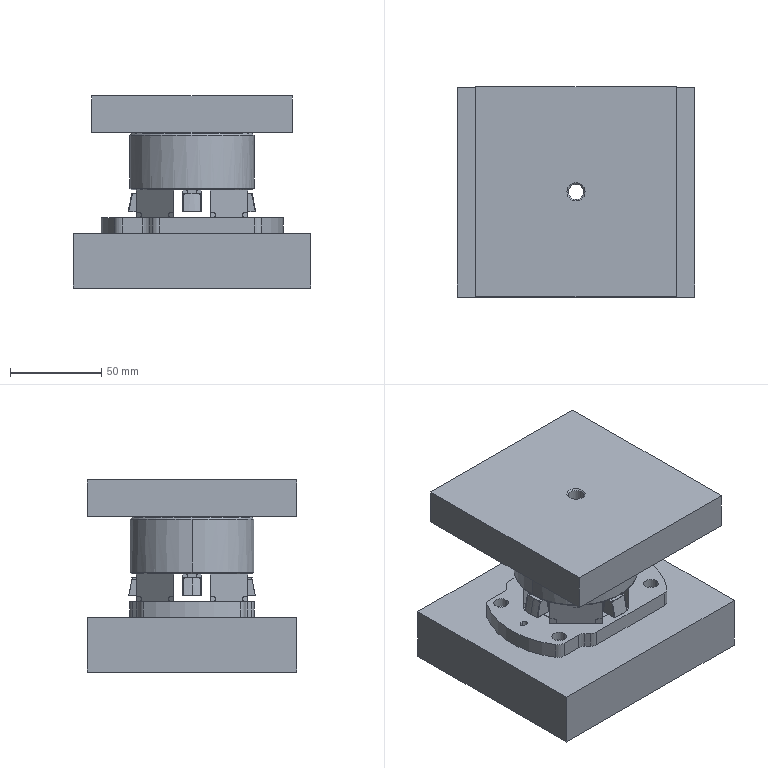NC program | NX | posted with a generic post | part box 130 x 115 x 105.2 mm
Lines 1 to 1155 of 3719:
N10 G17 G21 G94 G90
(PLANAR_MILL_COPY_4 , TOOL : D1.5R0)
N12 T16 M6
N14 G54
N16 G17 G0 G90 X-2.302 Y-5.448 S6000 M3
N18 G43 Z94. H16
N20 G94 G1 Z34.46 F5000.
N22 G41 X-3.284 Y-5.258 F1400. D16
N24 X-3.371 Y-5.25
N26 X-10.443
N28 X-12.2
N30 G2 X-13.95 Y-3.5 R1.75
N32 G3 X-14.2 Y-3.25 R0.25
N34 X-14.45 Y-3.5 R0.25
N36 G1 Y-4.929
N38 X-14.442 Y-5.016
N40 G40
N42 X-14.252 Y-5.998
N44 G0 Z37.71
N46 X-2.302 Y-5.448
N48 G1 Z34.21 F5000.
N50 G41 X-3.284 Y-5.258 F1400.
N52 X-3.371 Y-5.25
N54 X-10.443
N56 X-12.2
N58 G2 X-13.95 Y-3.5 R1.75
N60 G3 X-14.2 Y-3.25 R0.25
N62 X-14.45 Y-3.5 R0.25
N64 G1 Y-4.929
N66 X-14.442 Y-5.016
N68 G40
N70 X-14.252 Y-5.998
N72 G0 Z37.71
N74 X-2.302 Y-5.448
N76 G1 Z33.96 F5000.
N78 G41 X-3.284 Y-5.258 F1400.
N80 X-3.371 Y-5.25
N82 X-10.443
N84 X-12.2
N86 G2 X-13.95 Y-3.5 R1.75
N88 G3 X-14.2 Y-3.25 R0.25
N90 X-14.45 Y-3.5 R0.25
N92 G1 Y-4.929
N94 X-14.442 Y-5.016
N96 G40
N98 X-14.252 Y-5.998
N100 G0 Z37.71
N102 X-2.302 Y-5.448
N104 G1 Z33.71 F5000.
N106 G41 X-3.284 Y-5.258 F1400.
N108 X-3.371 Y-5.25
N110 X-10.443
N112 X-12.2
N114 G2 X-13.95 Y-3.5 R1.75
N116 G3 X-14.2 Y-3.25 R0.25
N118 X-14.45 Y-3.5 R0.25
N120 G1 Y-4.929
N122 X-14.442 Y-5.016
N124 G40
N126 X-14.252 Y-5.998
N128 G0 Z37.71
N130 X-2.302 Y-5.448
N132 G1 Z33.46 F5000.
N134 G41 X-3.284 Y-5.258 F1400.
N136 X-3.371 Y-5.25
N138 X-10.443
N140 X-12.2
N142 G2 X-13.95 Y-3.5 R1.75
N144 G3 X-14.2 Y-3.25 R0.25
N146 X-14.45 Y-3.5 R0.25
N148 G1 Y-4.929
N150 X-14.442 Y-5.016
N152 G40
N154 X-14.252 Y-5.998
N156 G0 Z37.71
N158 X-2.302 Y-5.448
N160 G1 Z33.21 F5000.
N162 G41 X-3.284 Y-5.258 F1400.
N164 X-3.371 Y-5.25
N166 X-10.443
N168 X-12.2
N170 G2 X-13.95 Y-3.5 R1.75
N172 G3 X-14.2 Y-3.25 R0.25
N174 X-14.45 Y-3.5 R0.25
N176 G1 Y-4.929
N178 X-14.442 Y-5.016
N180 G40
N182 X-14.252 Y-5.998
N184 G0 Z37.71
N186 X-2.302 Y-5.448
N188 G1 Z32.96 F5000.
N190 G41 X-3.284 Y-5.258 F1400.
N192 X-3.371 Y-5.25
N194 X-10.443
N196 X-12.2
N198 G2 X-13.95 Y-3.5 R1.75
N200 G3 X-14.2 Y-3.25 R0.25
N202 X-14.45 Y-3.5 R0.25
N204 G1 Y-4.929
N206 X-14.442 Y-5.016
N208 G40
N210 X-14.252 Y-5.998
N212 G0 Z37.71
N214 X-2.302 Y-5.448
N216 G1 Z32.71 F5000.
N218 G41 X-3.284 Y-5.258 F1400.
N220 X-3.371 Y-5.25
N222 X-10.443
N224 X-12.2
N226 G2 X-13.95 Y-3.5 R1.75
N228 G3 X-14.2 Y-3.25 R0.25
N230 X-14.45 Y-3.5 R0.25
N232 G1 Y-4.929
N234 X-14.442 Y-5.016
N236 G40
N238 X-14.252 Y-5.998
N240 G0 Z37.71
N242 X-2.302 Y-5.448
N244 G1 Z32.46 F5000.
N246 G41 X-3.284 Y-5.258 F1400.
N248 X-3.371 Y-5.25
N250 X-10.443
N252 X-12.2
N254 G2 X-13.95 Y-3.5 R1.75
N256 G3 X-14.2 Y-3.25 R0.25
N258 X-14.45 Y-3.5 R0.25
N260 G1 Y-4.929
N262 X-14.442 Y-5.016
N264 G40
N266 X-14.252 Y-5.998
N268 G0 Z37.71
N270 X-2.302 Y-5.448
N272 G1 Z32.21 F5000.
N274 G41 X-3.284 Y-5.258 F1400.
N276 X-3.371 Y-5.25
N278 X-10.443
N280 X-12.2
N282 G2 X-13.95 Y-3.5 R1.75
N284 G3 X-14.2 Y-3.25 R0.25
N286 X-14.45 Y-3.5 R0.25
N288 G1 Y-4.929
N290 X-14.442 Y-5.016
N292 G40
N294 X-14.252 Y-5.998
N296 G0 Z37.71
N298 X-2.302 Y-5.448
N300 G1 Z31.96 F5000.
N302 G41 X-3.284 Y-5.258 F1400.
N304 X-3.371 Y-5.25
N306 X-10.443
N308 X-12.2
N310 G2 X-13.95 Y-3.5 R1.75
N312 G3 X-14.2 Y-3.25 R0.25
N314 X-14.45 Y-3.5 R0.25
N316 G1 Y-4.929
N318 X-14.442 Y-5.016
N320 G40
N322 X-14.252 Y-5.998
N324 G0 Z37.71
N326 X-2.302 Y-5.448
N328 G1 Z31.71 F5000.
N330 G41 X-3.284 Y-5.258 F1400.
N332 X-3.371 Y-5.25
N334 X-10.443
N336 X-12.2
N338 G2 X-13.95 Y-3.5 R1.75
N340 G3 X-14.2 Y-3.25 R0.25
N342 X-14.45 Y-3.5 R0.25
N344 G1 Y-4.929
N346 X-14.442 Y-5.016
N348 G40
N350 X-14.252 Y-5.998
N352 G0 Z37.71
N354 X-2.302 Y-5.448
N356 G1 Z31.46 F5000.
N358 G41 X-3.284 Y-5.258 F1400.
N360 X-3.371 Y-5.25
N362 X-10.443
N364 X-12.2
N366 G2 X-13.95 Y-3.5 R1.75
N368 G3 X-14.2 Y-3.25 R0.25
N370 X-14.45 Y-3.5 R0.25
N372 G1 Y-4.929
N374 X-14.442 Y-5.016
N376 G40
N378 X-14.252 Y-5.998
N380 G0 Z37.71
N382 X-2.302 Y-5.448
N384 G1 Z31.21 F5000.
N386 G41 X-3.284 Y-5.258 F1400.
N388 X-3.371 Y-5.25
N390 X-10.443
N392 X-12.2
N394 G2 X-13.95 Y-3.5 R1.75
N396 G3 X-14.2 Y-3.25 R0.25
N398 X-14.45 Y-3.5 R0.25
N400 G1 Y-4.929
N402 X-14.442 Y-5.016
N404 G40
N406 X-14.252 Y-5.998
N408 G0 Z37.71
N410 X-2.302 Y-5.448
N412 G1 Z30.96 F5000.
N414 G41 X-3.284 Y-5.258 F1400.
N416 X-3.371 Y-5.25
N418 X-10.443
N420 X-12.2
N422 G2 X-13.95 Y-3.5 R1.75
N424 G3 X-14.2 Y-3.25 R0.25
N426 X-14.45 Y-3.5 R0.25
N428 G1 Y-4.929
N430 X-14.442 Y-5.016
N432 G40
N434 X-14.252 Y-5.998
N436 G0 Z37.71
N438 X-2.302 Y-5.448
N440 G1 Z30.71 F5000.
N442 G41 X-3.284 Y-5.258 F1400.
N444 X-3.371 Y-5.25
N446 X-10.443
N448 X-12.2
N450 G2 X-13.95 Y-3.5 R1.75
N452 G3 X-14.2 Y-3.25 R0.25
N454 X-14.45 Y-3.5 R0.25
N456 G1 Y-4.929
N458 X-14.442 Y-5.016
N460 G40
N462 X-14.252 Y-5.998
N464 G0 Z37.71
N466 X-2.302 Y-5.448
N468 G1 Z30.46 F5000.
N470 G41 X-3.284 Y-5.258 F1400.
N472 X-3.371 Y-5.25
N474 X-10.443
N476 X-12.2
N478 G2 X-13.95 Y-3.5 R1.75
N480 G3 X-14.2 Y-3.25 R0.25
N482 X-14.45 Y-3.5 R0.25
N484 G1 Y-4.929
N486 X-14.442 Y-5.016
N488 G40
N490 X-14.252 Y-5.998
N492 G0 Z37.71
N494 X-2.302 Y-5.448
N496 G1 Z30.21 F5000.
N498 G41 X-3.284 Y-5.258 F1400.
N500 X-3.371 Y-5.25
N502 X-10.443
N504 X-12.2
N506 G2 X-13.95 Y-3.5 R1.75
N508 G3 X-14.2 Y-3.25 R0.25
N510 X-14.45 Y-3.5 R0.25
N512 G1 Y-4.929
N514 X-14.442 Y-5.016
N516 G40
N518 X-14.252 Y-5.998
N520 G0 Z37.71
N522 X-2.302 Y-5.448
N524 G1 Z29.96 F5000.
N526 G41 X-3.284 Y-5.258 F1400.
N528 X-3.371 Y-5.25
N530 X-10.443
N532 X-12.2
N534 G2 X-13.95 Y-3.5 R1.75
N536 G3 X-14.2 Y-3.25 R0.25
N538 X-14.45 Y-3.5 R0.25
N540 G1 Y-4.929
N542 X-14.442 Y-5.016
N544 G40
N546 X-14.252 Y-5.998
N548 G0 Z37.71
N550 X-2.302 Y-5.448
N552 G1 Z29.71 F5000.
N554 G41 X-3.284 Y-5.258 F1400.
N556 X-3.371 Y-5.25
N558 X-10.443
N560 X-12.2
N562 G2 X-13.95 Y-3.5 R1.75
N564 G3 X-14.2 Y-3.25 R0.25
N566 X-14.45 Y-3.5 R0.25
N568 G1 Y-4.929
N570 X-14.442 Y-5.016
N572 G40
N574 X-14.252 Y-5.998
N576 G0 Z37.71
N578 X-2.302 Y-5.448
N580 G1 Z29.46 F5000.
N582 G41 X-3.284 Y-5.258 F1400.
N584 X-3.371 Y-5.25
N586 X-10.443
N588 X-12.2
N590 G2 X-13.95 Y-3.5 R1.75
N592 G3 X-14.2 Y-3.25 R0.25
N594 X-14.45 Y-3.5 R0.25
N596 G1 Y-4.929
N598 X-14.442 Y-5.016
N600 G40
N602 X-14.252 Y-5.998
N604 G0 Z37.71
N606 X-2.302 Y-5.448
N608 G1 Z29.21 F5000.
N610 G41 X-3.284 Y-5.258 F1400.
N612 X-3.371 Y-5.25
N614 X-10.443
N616 X-12.2
N618 G2 X-13.95 Y-3.5 R1.75
N620 G3 X-14.2 Y-3.25 R0.25
N622 X-14.45 Y-3.5 R0.25
N624 G1 Y-4.929
N626 X-14.442 Y-5.016
N628 G40
N630 X-14.252 Y-5.998
N632 G0 Z37.71
N634 X-2.302 Y-5.448
N636 G1 Z28.96 F5000.
N638 G41 X-3.284 Y-5.258 F1400.
N640 X-3.371 Y-5.25
N642 X-10.443
N644 X-12.2
N646 G2 X-13.95 Y-3.5 R1.75
N648 G3 X-14.2 Y-3.25 R0.25
N650 X-14.45 Y-3.5 R0.25
N652 G1 Y-4.929
N654 X-14.442 Y-5.016
N656 G40
N658 X-14.252 Y-5.998
N660 G0 Z37.71
N662 X-2.302 Y-5.448
N664 G1 Z28.71 F5000.
N666 G41 X-3.284 Y-5.258 F1400.
N668 X-3.371 Y-5.25
N670 X-10.443
N672 X-12.2
N674 G2 X-13.95 Y-3.5 R1.75
N676 G3 X-14.2 Y-3.25 R0.25
N678 X-14.45 Y-3.5 R0.25
N680 G1 Y-4.929
N682 X-14.442 Y-5.016
N684 G40
N686 X-14.252 Y-5.998
N688 G0 Z37.71
N690 X-2.302 Y-5.448
N692 G1 Z28.46 F5000.
N694 G41 X-3.284 Y-5.258 F1400.
N696 X-3.371 Y-5.25
N698 X-10.443
N700 X-12.2
N702 G2 X-13.95 Y-3.5 R1.75
N704 G3 X-14.2 Y-3.25 R0.25
N706 X-14.45 Y-3.5 R0.25
N708 G1 Y-4.929
N710 X-14.442 Y-5.016
N712 G40
N714 X-14.252 Y-5.998
N716 G0 Z37.71
N718 X-2.302 Y-5.448
N720 G1 Z28.21 F5000.
N722 G41 X-3.284 Y-5.258 F1400.
N724 X-3.371 Y-5.25
N726 X-10.443
N728 X-12.2
N730 G2 X-13.95 Y-3.5 R1.75
N732 G3 X-14.2 Y-3.25 R0.25
N734 X-14.45 Y-3.5 R0.25
N736 G1 Y-4.929
N738 X-14.442 Y-5.016
N740 G40
N742 X-14.252 Y-5.998
N744 G0 Z37.71
N746 X-2.302 Y-5.448
N748 G1 Z27.96 F5000.
N750 G41 X-3.284 Y-5.258 F1400.
N752 X-3.371 Y-5.25
N754 X-10.443
N756 X-12.2
N758 G2 X-13.95 Y-3.5 R1.75
N760 G3 X-14.2 Y-3.25 R0.25
N762 X-14.45 Y-3.5 R0.25
N764 G1 Y-4.929
N766 X-14.442 Y-5.016
N768 G40
N770 X-14.252 Y-5.998
N772 G0 Z37.71
N774 X-2.302 Y-5.448
N776 G1 Z27.71 F5000.
N778 G41 X-3.284 Y-5.258 F1400.
N780 X-3.371 Y-5.25
N782 X-10.443
N784 X-12.2
N786 G2 X-13.95 Y-3.5 R1.75
N788 G3 X-14.2 Y-3.25 R0.25
N790 X-14.45 Y-3.5 R0.25
N792 G1 Y-4.929
N794 X-14.442 Y-5.016
N796 G40
N798 X-14.252 Y-5.998
N800 G0 Z37.71
N802 X-2.302 Y-5.448
N804 G1 Z27.46 F5000.
N806 G41 X-3.284 Y-5.258 F1400.
N808 X-3.371 Y-5.25
N810 X-10.443
N812 X-12.2
N814 G2 X-13.95 Y-3.5 R1.75
N816 G3 X-14.2 Y-3.25 R0.25
N818 X-14.45 Y-3.5 R0.25
N820 G1 Y-4.929
N822 X-14.442 Y-5.016
N824 G40
N826 X-14.252 Y-5.998
N828 G0 Z37.71
N830 X-2.302 Y-5.448
N832 G1 Z27.21 F5000.
N834 G41 X-3.284 Y-5.258 F1400.
N836 X-3.371 Y-5.25
N838 X-10.443
N840 X-12.2
N842 G2 X-13.95 Y-3.5 R1.75
N844 G3 X-14.2 Y-3.25 R0.25
N846 X-14.45 Y-3.5 R0.25
N848 G1 Y-4.929
N850 X-14.442 Y-5.016
N852 G40
N854 X-14.252 Y-5.998
N856 G0 Z37.71
N858 X-2.302 Y-5.448
N860 G1 Z26.96 F5000.
N862 G41 X-3.284 Y-5.258 F1400.
N864 X-3.371 Y-5.25
N866 X-10.443
N868 X-12.2
N870 G2 X-13.95 Y-3.5 R1.75
N872 G3 X-14.2 Y-3.25 R0.25
N874 X-14.45 Y-3.5 R0.25
N876 G1 Y-4.929
N878 X-14.442 Y-5.016
N880 G40
N882 X-14.252 Y-5.998
N884 G0 Z37.71
N886 X-2.302 Y-5.448
N888 G1 Z26.71 F5000.
N890 G41 X-3.284 Y-5.258 F1400.
N892 X-3.371 Y-5.25
N894 X-10.443
N896 X-12.2
N898 G2 X-13.95 Y-3.5 R1.75
N900 G3 X-14.2 Y-3.25 R0.25
N902 X-14.45 Y-3.5 R0.25
N904 G1 Y-4.929
N906 X-14.442 Y-5.016
N908 G40
N910 X-14.252 Y-5.998
N912 G0 Z37.71
N914 X-2.302 Y-5.448
N916 G1 Z26.55 F5000.
N918 G41 X-3.284 Y-5.258 F1400.
N920 X-3.371 Y-5.25
N922 X-10.443
N924 X-12.2
N926 G2 X-13.95 Y-3.5 R1.75
N928 G3 X-14.2 Y-3.25 R0.25
N930 X-14.45 Y-3.5 R0.25
N932 G1 Y-4.929
N934 X-14.442 Y-5.016
N936 G40
N938 X-14.252 Y-5.998
N940 G0 Z37.71
N942 Y5.998
N944 G1 Z34.46 F5000.
N946 G41 X-14.442 Y5.016 F1400.
N948 X-14.45 Y4.929
N950 Y3.5
N952 G3 X-14.2 Y3.25 R0.25
N954 X-13.95 Y3.5 R0.25
N956 G2 X-12.2 Y5.25 R1.75
N958 G1 X-11.317
N960 X-3.371
N962 X-3.284 Y5.258
N964 G40
N966 X-2.302 Y5.448
N968 G0 Z37.71
N970 X-14.252 Y5.998
N972 G1 Z34.21 F5000.
N974 G41 X-14.442 Y5.016 F1400.
N976 X-14.45 Y4.929
N978 Y3.5
N980 G3 X-14.2 Y3.25 R0.25
N982 X-13.95 Y3.5 R0.25
N984 G2 X-12.2 Y5.25 R1.75
N986 G1 X-11.317
N988 X-3.371
N990 X-3.284 Y5.258
N992 G40
N994 X-2.302 Y5.448
N996 G0 Z37.71
N998 X-14.252 Y5.998
N1000 G1 Z33.96 F5000.
N1002 G41 X-14.442 Y5.016 F1400.
N1004 X-14.45 Y4.929
N1006 Y3.5
N1008 G3 X-14.2 Y3.25 R0.25
N1010 X-13.95 Y3.5 R0.25
N1012 G2 X-12.2 Y5.25 R1.75
N1014 G1 X-11.317
N1016 X-3.371
N1018 X-3.284 Y5.258
N1020 G40
N1022 X-2.302 Y5.448
N1024 G0 Z37.71
N1026 X-14.252 Y5.998
N1028 G1 Z33.71 F5000.
N1030 G41 X-14.442 Y5.016 F1400.
N1032 X-14.45 Y4.929
N1034 Y3.5
N1036 G3 X-14.2 Y3.25 R0.25
N1038 X-13.95 Y3.5 R0.25
N1040 G2 X-12.2 Y5.25 R1.75
N1042 G1 X-11.317
N1044 X-3.371
N1046 X-3.284 Y5.258
N1048 G40
N1050 X-2.302 Y5.448
N1052 G0 Z37.71
N1054 X-14.252 Y5.998
N1056 G1 Z33.46 F5000.
N1058 G41 X-14.442 Y5.016 F1400.
N1060 X-14.45 Y4.929
N1062 Y3.5
N1064 G3 X-14.2 Y3.25 R0.25
N1066 X-13.95 Y3.5 R0.25
N1068 G2 X-12.2 Y5.25 R1.75
N1070 G1 X-11.317
N1072 X-3.371
N1074 X-3.284 Y5.258
N1076 G40
N1078 X-2.302 Y5.448
N1080 G0 Z37.71
N1082 X-14.252 Y5.998
N1084 G1 Z33.21 F5000.
N1086 G41 X-14.442 Y5.016 F1400.
N1088 X-14.45 Y4.929
N1090 Y3.5
N1092 G3 X-14.2 Y3.25 R0.25
N1094 X-13.95 Y3.5 R0.25
N1096 G2 X-12.2 Y5.25 R1.75
N1098 G1 X-11.317
N1100 X-3.371
N1102 X-3.284 Y5.258
N1104 G40
N1106 X-2.302 Y5.448
N1108 G0 Z37.71
N1110 X-14.252 Y5.998
N1112 G1 Z32.96 F5000.
N1114 G41 X-14.442 Y5.016 F1400.
N1116 X-14.45 Y4.929
N1118 Y3.5
N1120 G3 X-14.2 Y3.25 R0.25
N1122 X-13.95 Y3.5 R0.25
N1124 G2 X-12.2 Y5.25 R1.75
N1126 G1 X-11.317
N1128 X-3.371
N1130 X-3.284 Y5.258
N1132 G40
N1134 X-2.302 Y5.448
N1136 G0 Z37.71
N1138 X-14.252 Y5.998
N1140 G1 Z32.71 F5000.
N1142 G41 X-14.442 Y5.016 F1400.
N1144 X-14.45 Y4.929
N1146 Y3.5
N1148 G3 X-14.2 Y3.25 R0.25
N1150 X-13.95 Y3.5 R0.25
N1152 G2 X-12.2 Y5.25 R1.75
N1154 G1 X-11.317
N1156 X-3.371
N1158 X-3.284 Y5.258
N1160 G40
N1162 X-2.302 Y5.448
N1164 G0 Z37.71
N1166 X-14.252 Y5.998
N1168 G1 Z32.46 F5000.
N1170 G41 X-14.442 Y5.016 F1400.
N1172 X-14.45 Y4.929
N1174 Y3.5
N1176 G3 X-14.2 Y3.25 R0.25
N1178 X-13.95 Y3.5 R0.25
N1180 G2 X-12.2 Y5.25 R1.75
N1182 G1 X-11.317
N1184 X-3.371
N1186 X-3.284 Y5.258
N1188 G40
N1190 X-2.302 Y5.448
N1192 G0 Z37.71
N1194 X-14.252 Y5.998
N1196 G1 Z32.21 F5000.
N1198 G41 X-14.442 Y5.016 F1400.
N1200 X-14.45 Y4.929
N1202 Y3.5
N1204 G3 X-14.2 Y3.25 R0.25
N1206 X-13.95 Y3.5 R0.25
N1208 G2 X-12.2 Y5.25 R1.75
N1210 G1 X-11.317
N1212 X-3.371
N1214 X-3.284 Y5.258
N1216 G40
N1218 X-2.302 Y5.448
N1220 G0 Z37.71
N1222 X-14.252 Y5.998
N1224 G1 Z31.96 F5000.
N1226 G41 X-14.442 Y5.016 F1400.
N1228 X-14.45 Y4.929
N1230 Y3.5
N1232 G3 X-14.2 Y3.25 R0.25
N1234 X-13.95 Y3.5 R0.25
N1236 G2 X-12.2 Y5.25 R1.75
N1238 G1 X-11.317
N1240 X-3.371
N1242 X-3.284 Y5.258
N1244 G40
N1246 X-2.302 Y5.448
N1248 G0 Z37.71
N1250 X-14.252 Y5.998
N1252 G1 Z31.71 F5000.
N1254 G41 X-14.442 Y5.016 F1400.
N1256 X-14.45 Y4.929
N1258 Y3.5
N1260 G3 X-14.2 Y3.25 R0.25
N1262 X-13.95 Y3.5 R0.25
N1264 G2 X-12.2 Y5.25 R1.75
N1266 G1 X-11.317
N1268 X-3.371
N1270 X-3.284 Y5.258
N1272 G40
N1274 X-2.302 Y5.448
N1276 G0 Z37.71
N1278 X-14.252 Y5.998
N1280 G1 Z31.46 F5000.
N1282 G41 X-14.442 Y5.016 F1400.
N1284 X-14.45 Y4.929
N1286 Y3.5
N1288 G3 X-14.2 Y3.25 R0.25
N1290 X-13.95 Y3.5 R0.25
N1292 G2 X-12.2 Y5.25 R1.75
N1294 G1 X-11.317
N1296 X-3.371
N1298 X-3.284 Y5.258
N1300 G40
N1302 X-2.302 Y5.448
N1304 G0 Z37.71
N1306 X-14.252 Y5.998
N1308 G1 Z31.21 F5000.
N1310 G41 X-14.442 Y5.016 F1400.
N1312 X-14.45 Y4.929
N1314 Y3.5
N1316 G3 X-14.2 Y3.25 R0.25
N1318 X-13.95 Y3.5 R0.25
N1320 G2 X-12.2 Y5.25 R1.75
N1322 G1 X-11.317
N1324 X-3.371
N1326 X-3.284 Y5.258
N1328 G40
N1330 X-2.302 Y5.448
N1332 G0 Z37.71
N1334 X-14.252 Y5.998
N1336 G1 Z30.96 F5000.
N1338 G41 X-14.442 Y5.016 F1400.
N1340 X-14.45 Y4.929
N1342 Y3.5
N1344 G3 X-14.2 Y3.25 R0.25
N1346 X-13.95 Y3.5 R0.25
N1348 G2 X-12.2 Y5.25 R1.75
N1350 G1 X-11.317
N1352 X-3.371
N1354 X-3.284 Y5.258
N1356 G40
N1358 X-2.302 Y5.448
N1360 G0 Z37.71
N1362 X-14.252 Y5.998
N1364 G1 Z30.71 F5000.
N1366 G41 X-14.442 Y5.016 F1400.
N1368 X-14.45 Y4.929
N1370 Y3.5
N1372 G3 X-14.2 Y3.25 R0.25
N1374 X-13.95 Y3.5 R0.25
N1376 G2 X-12.2 Y5.25 R1.75
N1378 G1 X-11.317
N1380 X-3.371
N1382 X-3.284 Y5.258
N1384 G40
N1386 X-2.302 Y5.448
N1388 G0 Z37.71
N1390 X-14.252 Y5.998
N1392 G1 Z30.46 F5000.
N1394 G41 X-14.442 Y5.016 F1400.
N1396 X-14.45 Y4.929
N1398 Y3.5
N1400 G3 X-14.2 Y3.25 R0.25
N1402 X-13.95 Y3.5 R0.25
N1404 G2 X-12.2 Y5.25 R1.75
N1406 G1 X-11.317
N1408 X-3.371
N1410 X-3.284 Y5.258
N1412 G40
N1414 X-2.302 Y5.448
N1416 G0 Z37.71
N1418 X-14.252 Y5.998
N1420 G1 Z30.21 F5000.
N1422 G41 X-14.442 Y5.016 F1400.
N1424 X-14.45 Y4.929
N1426 Y3.5
N1428 G3 X-14.2 Y3.25 R0.25
N1430 X-13.95 Y3.5 R0.25
N1432 G2 X-12.2 Y5.25 R1.75
N1434 G1 X-11.317
N1436 X-3.371
N1438 X-3.284 Y5.258
N1440 G40
N1442 X-2.302 Y5.448
N1444 G0 Z37.71
N1446 X-14.252 Y5.998
N1448 G1 Z29.96 F5000.
N1450 G41 X-14.442 Y5.016 F1400.
N1452 X-14.45 Y4.929
N1454 Y3.5
N1456 G3 X-14.2 Y3.25 R0.25
N1458 X-13.95 Y3.5 R0.25
N1460 G2 X-12.2 Y5.25 R1.75
N1462 G1 X-11.317
N1464 X-3.371
N1466 X-3.284 Y5.258
N1468 G40
N1470 X-2.302 Y5.448
N1472 G0 Z37.71
N1474 X-14.252 Y5.998
N1476 G1 Z29.71 F5000.
N1478 G41 X-14.442 Y5.016 F1400.
N1480 X-14.45 Y4.929
N1482 Y3.5
N1484 G3 X-14.2 Y3.25 R0.25
N1486 X-13.95 Y3.5 R0.25
N1488 G2 X-12.2 Y5.25 R1.75
N1490 G1 X-11.317
N1492 X-3.371
N1494 X-3.284 Y5.258
N1496 G40
N1498 X-2.302 Y5.448
N1500 G0 Z37.71
N1502 X-14.252 Y5.998
N1504 G1 Z29.46 F5000.
N1506 G41 X-14.442 Y5.016 F1400.
N1508 X-14.45 Y4.929
N1510 Y3.5
N1512 G3 X-14.2 Y3.25 R0.25
N1514 X-13.95 Y3.5 R0.25
N1516 G2 X-12.2 Y5.25 R1.75
N1518 G1 X-11.317
N1520 X-3.371
N1522 X-3.284 Y5.258
N1524 G40
N1526 X-2.302 Y5.448
N1528 G0 Z37.71
N1530 X-14.252 Y5.998
N1532 G1 Z29.21 F5000.
N1534 G41 X-14.442 Y5.016 F1400.
N1536 X-14.45 Y4.929
N1538 Y3.5
N1540 G3 X-14.2 Y3.25 R0.25
N1542 X-13.95 Y3.5 R0.25
N1544 G2 X-12.2 Y5.25 R1.75
N1546 G1 X-11.317
N1548 X-3.371
N1550 X-3.284 Y5.258
N1552 G40
N1554 X-2.302 Y5.448
N1556 G0 Z37.71
N1558 X-14.252 Y5.998
N1560 G1 Z28.96 F5000.
N1562 G41 X-14.442 Y5.016 F1400.
N1564 X-14.45 Y4.929
N1566 Y3.5
N1568 G3 X-14.2 Y3.25 R0.25
N1570 X-13.95 Y3.5 R0.25
N1572 G2 X-12.2 Y5.25 R1.75
N1574 G1 X-11.317
N1576 X-3.371
N1578 X-3.284 Y5.258
N1580 G40
N1582 X-2.302 Y5.448
N1584 G0 Z37.71
N1586 X-14.252 Y5.998
N1588 G1 Z28.71 F5000.
N1590 G41 X-14.442 Y5.016 F1400.
N1592 X-14.45 Y4.929
N1594 Y3.5
N1596 G3 X-14.2 Y3.25 R0.25
N1598 X-13.95 Y3.5 R0.25
N1600 G2 X-12.2 Y5.25 R1.75
N1602 G1 X-11.317
N1604 X-3.371
N1606 X-3.284 Y5.258
N1608 G40
N1610 X-2.302 Y5.448
N1612 G0 Z37.71
N1614 X-14.252 Y5.998
N1616 G1 Z28.46 F5000.
N1618 G41 X-14.442 Y5.016 F1400.
N1620 X-14.45 Y4.929
N1622 Y3.5
N1624 G3 X-14.2 Y3.25 R0.25
N1626 X-13.95 Y3.5 R0.25
N1628 G2 X-12.2 Y5.25 R1.75
N1630 G1 X-11.317
N1632 X-3.371
N1634 X-3.284 Y5.258
N1636 G40
N1638 X-2.302 Y5.448
N1640 G0 Z37.71
N1642 X-14.252 Y5.998
N1644 G1 Z28.21 F5000.
N1646 G41 X-14.442 Y5.016 F1400.
N1648 X-14.45 Y4.929
N1650 Y3.5
N1652 G3 X-14.2 Y3.25 R0.25
N1654 X-13.95 Y3.5 R0.25
N1656 G2 X-12.2 Y5.25 R1.75
N1658 G1 X-11.317
N1660 X-3.371
N1662 X-3.284 Y5.258
N1664 G40
N1666 X-2.302 Y5.448
N1668 G0 Z37.71
N1670 X-14.252 Y5.998
N1672 G1 Z27.96 F5000.
N1674 G41 X-14.442 Y5.016 F1400.
N1676 X-14.45 Y4.929
N1678 Y3.5
N1680 G3 X-14.2 Y3.25 R0.25
N1682 X-13.95 Y3.5 R0.25
N1684 G2 X-12.2 Y5.25 R1.75
N1686 G1 X-11.317
N1688 X-3.371
N1690 X-3.284 Y5.258
N1692 G40
N1694 X-2.302 Y5.448
N1696 G0 Z37.71
N1698 X-14.252 Y5.998
N1700 G1 Z27.71 F5000.
N1702 G41 X-14.442 Y5.016 F1400.
N1704 X-14.45 Y4.929
N1706 Y3.5
N1708 G3 X-14.2 Y3.25 R0.25
N1710 X-13.95 Y3.5 R0.25
N1712 G2 X-12.2 Y5.25 R1.75
N1714 G1 X-11.317
N1716 X-3.371
N1718 X-3.284 Y5.258
N1720 G40
N1722 X-2.302 Y5.448
N1724 G0 Z37.71
N1726 X-14.252 Y5.998
N1728 G1 Z27.46 F5000.
N1730 G41 X-14.442 Y5.016 F1400.
N1732 X-14.45 Y4.929
N1734 Y3.5
N1736 G3 X-14.2 Y3.25 R0.25
N1738 X-13.95 Y3.5 R0.25
N1740 G2 X-12.2 Y5.25 R1.75
N1742 G1 X-11.317
N1744 X-3.371
N1746 X-3.284 Y5.258
N1748 G40
N1750 X-2.302 Y5.448
N1752 G0 Z37.71
N1754 X-14.252 Y5.998
N1756 G1 Z27.21 F5000.
N1758 G41 X-14.442 Y5.016 F1400.
N1760 X-14.45 Y4.929
N1762 Y3.5
N1764 G3 X-14.2 Y3.25 R0.25
N1766 X-13.95 Y3.5 R0.25
N1768 G2 X-12.2 Y5.25 R1.75
N1770 G1 X-11.317
N1772 X-3.371
N1774 X-3.284 Y5.258
N1776 G40
N1778 X-2.302 Y5.448
N1780 G0 Z37.71
N1782 X-14.252 Y5.998
N1784 G1 Z26.96 F5000.
N1786 G41 X-14.442 Y5.016 F1400.
N1788 X-14.45 Y4.929
N1790 Y3.5
N1792 G3 X-14.2 Y3.25 R0.25
N1794 X-13.95 Y3.5 R0.25
N1796 G2 X-12.2 Y5.25 R1.75
N1798 G1 X-11.317
N1800 X-3.371
N1802 X-3.284 Y5.258
N1804 G40
N1806 X-2.302 Y5.448
N1808 G0 Z37.71
N1810 X-14.252 Y5.998
N1812 G1 Z26.71 F5000.
N1814 G41 X-14.442 Y5.016 F1400.
N1816 X-14.45 Y4.929
N1818 Y3.5
N1820 G3 X-14.2 Y3.25 R0.25
N1822 X-13.95 Y3.5 R0.25
N1824 G2 X-12.2 Y5.25 R1.75
N1826 G1 X-11.317
N1828 X-3.371
N1830 X-3.284 Y5.258
N1832 G40
N1834 X-2.302 Y5.448
N1836 G0 Z37.71
N1838 X-14.252 Y5.998
N1840 G1 Z26.55 F5000.
N1842 G41 X-14.442 Y5.016 F1400.
N1844 X-14.45 Y4.929
N1846 Y3.5
N1848 G3 X-14.2 Y3.25 R0.25
N1850 X-13.95 Y3.5 R0.25
N1852 G2 X-12.2 Y5.25 R1.75
N1854 G1 X-11.317
N1856 X-3.371
N1858 X-3.284 Y5.258
N1860 G40
N1862 X-2.302 Y5.448
N1864 G0 Z94.
(PLANAR_MILL_COPY_4_COPY , TOOL : D1.5R0)
N1866 G18 X-2.302 Z-5.448
N1868 Y-94.
N1870 G1 Y-34.46 F5000.
N1872 G41 X-3.284 Z-5.258 F1400.
N1874 X-3.371 Z-5.25
N1876 X-10.443
N1878 X-12.2
N1880 G3 X-13.95 Z-3.5 R1.75
N1882 G2 X-14.2 Z-3.25 R0.25
N1884 X-14.45 Z-3.5 R0.25
N1886 G1 Z-4.929
N1888 X-14.442 Z-5.016
N1890 G40
N1892 X-14.252 Z-5.998
N1894 G0 Y-37.71
N1896 X-2.302 Z-5.448
N1898 G1 Y-34.21 F5000.
N1900 G41 X-3.284 Z-5.258 F1400.
N1902 X-3.371 Z-5.25
N1904 X-10.443
N1906 X-12.2
N1908 G3 X-13.95 Z-3.5 R1.75
N1910 G2 X-14.2 Z-3.25 R0.25
N1912 X-14.45 Z-3.5 R0.25
N1914 G1 Z-4.929
N1916 X-14.442 Z-5.016
N1918 G40
N1920 X-14.252 Z-5.998
N1922 G0 Y-37.71
N1924 X-2.302 Z-5.448
N1926 G1 Y-33.96 F5000.
N1928 G41 X-3.284 Z-5.258 F1400.
N1930 X-3.371 Z-5.25
N1932 X-10.443
N1934 X-12.2
N1936 G3 X-13.95 Z-3.5 R1.75
N1938 G2 X-14.2 Z-3.25 R0.25
N1940 X-14.45 Z-3.5 R0.25
N1942 G1 Z-4.929
N1944 X-14.442 Z-5.016
N1946 G40
N1948 X-14.252 Z-5.998
N1950 G0 Y-37.71
N1952 X-2.302 Z-5.448
N1954 G1 Y-33.71 F5000.
N1956 G41 X-3.284 Z-5.258 F1400.
N1958 X-3.371 Z-5.25
N1960 X-10.443
N1962 X-12.2
N1964 G3 X-13.95 Z-3.5 R1.75
N1966 G2 X-14.2 Z-3.25 R0.25
N1968 X-14.45 Z-3.5 R0.25
N1970 G1 Z-4.929
N1972 X-14.442 Z-5.016
N1974 G40
N1976 X-14.252 Z-5.998
N1978 G0 Y-37.71
N1980 X-2.302 Z-5.448
N1982 G1 Y-33.46 F5000.
N1984 G41 X-3.284 Z-5.258 F1400.
N1986 X-3.371 Z-5.25
N1988 X-10.443
N1990 X-12.2
N1992 G3 X-13.95 Z-3.5 R1.75
N1994 G2 X-14.2 Z-3.25 R0.25
N1996 X-14.45 Z-3.5 R0.25
N1998 G1 Z-4.929
N2000 X-14.442 Z-5.016
N2002 G40
N2004 X-14.252 Z-5.998
N2006 G0 Y-37.71
N2008 X-2.302 Z-5.448
N2010 G1 Y-33.21 F5000.
N2012 G41 X-3.284 Z-5.258 F1400.
N2014 X-3.371 Z-5.25
N2016 X-10.443
N2018 X-12.2
N2020 G3 X-13.95 Z-3.5 R1.75
N2022 G2 X-14.2 Z-3.25 R0.25
N2024 X-14.45 Z-3.5 R0.25
N2026 G1 Z-4.929
N2028 X-14.442 Z-5.016
N2030 G40
N2032 X-14.252 Z-5.998
N2034 G0 Y-37.71
N2036 X-2.302 Z-5.448
N2038 G1 Y-32.96 F5000.
N2040 G41 X-3.284 Z-5.258 F1400.
N2042 X-3.371 Z-5.25
N2044 X-10.443
N2046 X-12.2
N2048 G3 X-13.95 Z-3.5 R1.75
N2050 G2 X-14.2 Z-3.25 R0.25
N2052 X-14.45 Z-3.5 R0.25
N2054 G1 Z-4.929
N2056 X-14.442 Z-5.016
N2058 G40
N2060 X-14.252 Z-5.998
N2062 G0 Y-37.71
N2064 X-2.302 Z-5.448
N2066 G1 Y-32.71 F5000.
N2068 G41 X-3.284 Z-5.258 F1400.
N2070 X-3.371 Z-5.25
N2072 X-10.443
N2074 X-12.2
N2076 G3 X-13.95 Z-3.5 R1.75
N2078 G2 X-14.2 Z-3.25 R0.25
N2080 X-14.45 Z-3.5 R0.25
N2082 G1 Z-4.929
N2084 X-14.442 Z-5.016
N2086 G40
N2088 X-14.252 Z-5.998
N2090 G0 Y-37.71
N2092 X-2.302 Z-5.448
N2094 G1 Y-32.46 F5000.
N2096 G41 X-3.284 Z-5.258 F1400.
N2098 X-3.371 Z-5.25
N2100 X-10.443
N2102 X-12.2
N2104 G3 X-13.95 Z-3.5 R1.75
N2106 G2 X-14.2 Z-3.25 R0.25
N2108 X-14.45 Z-3.5 R0.25
N2110 G1 Z-4.929
N2112 X-14.442 Z-5.016
N2114 G40
N2116 X-14.252 Z-5.998
N2118 G0 Y-37.71
N2120 X-2.302 Z-5.448
N2122 G1 Y-32.21 F5000.
N2124 G41 X-3.284 Z-5.258 F1400.
N2126 X-3.371 Z-5.25
N2128 X-10.443
N2130 X-12.2
N2132 G3 X-13.95 Z-3.5 R1.75
N2134 G2 X-14.2 Z-3.25 R0.25
N2136 X-14.45 Z-3.5 R0.25
N2138 G1 Z-4.929
N2140 X-14.442 Z-5.016
N2142 G40
N2144 X-14.252 Z-5.998
N2146 G0 Y-37.71
N2148 X-2.302 Z-5.448
N2150 G1 Y-31.96 F5000.
N2152 G41 X-3.284 Z-5.258 F1400.
N2154 X-3.371 Z-5.25
N2156 X-10.443
N2158 X-12.2
N2160 G3 X-13.95 Z-3.5 R1.75
N2162 G2 X-14.2 Z-3.25 R0.25
N2164 X-14.45 Z-3.5 R0.25
N2166 G1 Z-4.929
N2168 X-14.442 Z-5.016
N2170 G40
N2172 X-14.252 Z-5.998
N2174 G0 Y-37.71
N2176 X-2.302 Z-5.448
N2178 G1 Y-31.71 F5000.
N2180 G41 X-3.284 Z-5.258 F1400.
N2182 X-3.371 Z-5.25
N2184 X-10.443
N2186 X-12.2
N2188 G3 X-13.95 Z-3.5 R1.75
N2190 G2 X-14.2 Z-3.25 R0.25
N2192 X-14.45 Z-3.5 R0.25
N2194 G1 Z-4.929
N2196 X-14.442 Z-5.016
N2198 G40
N2200 X-14.252 Z-5.998
N2202 G0 Y-37.71
N2204 X-2.302 Z-5.448
N2206 G1 Y-31.46 F5000.
N2208 G41 X-3.284 Z-5.258 F1400.
N2210 X-3.371 Z-5.25
N2212 X-10.443
N2214 X-12.2
N2216 G3 X-13.95 Z-3.5 R1.75
N2218 G2 X-14.2 Z-3.25 R0.25
N2220 X-14.45 Z-3.5 R0.25
N2222 G1 Z-4.929
N2224 X-14.442 Z-5.016
N2226 G40
N2228 X-14.252 Z-5.998
N2230 G0 Y-37.71
N2232 X-2.302 Z-5.448
N2234 G1 Y-31.21 F5000.
N2236 G41 X-3.284 Z-5.258 F1400.
N2238 X-3.371 Z-5.25
N2240 X-10.443
N2242 X-12.2
N2244 G3 X-13.95 Z-3.5 R1.75
N2246 G2 X-14.2 Z-3.25 R0.25
N2248 X-14.45 Z-3.5 R0.25
N2250 G1 Z-4.929
N2252 X-14.442 Z-5.016
N2254 G40
N2256 X-14.252 Z-5.998
N2258 G0 Y-37.71
N2260 X-2.302 Z-5.448
N2262 G1 Y-30.96 F5000.
N2264 G41 X-3.284 Z-5.258 F1400.
N2266 X-3.371 Z-5.25
N2268 X-10.443
N2270 X-12.2
N2272 G3 X-13.95 Z-3.5 R1.75
N2274 G2 X-14.2 Z-3.25 R0.25
N2276 X-14.45 Z-3.5 R0.25
N2278 G1 Z-4.929
N2280 X-14.442 Z-5.016
N2282 G40
N2284 X-14.252 Z-5.998
N2286 G0 Y-37.71
N2288 X-2.302 Z-5.448
N2290 G1 Y-30.71 F5000.
N2292 G41 X-3.284 Z-5.258 F1400.
N2294 X-3.371 Z-5.25
N2296 X-10.443
N2298 X-12.2
N2300 G3 X-13.95 Z-3.5 R1.75
N2302 G2 X-14.2 Z-3.25 R0.25